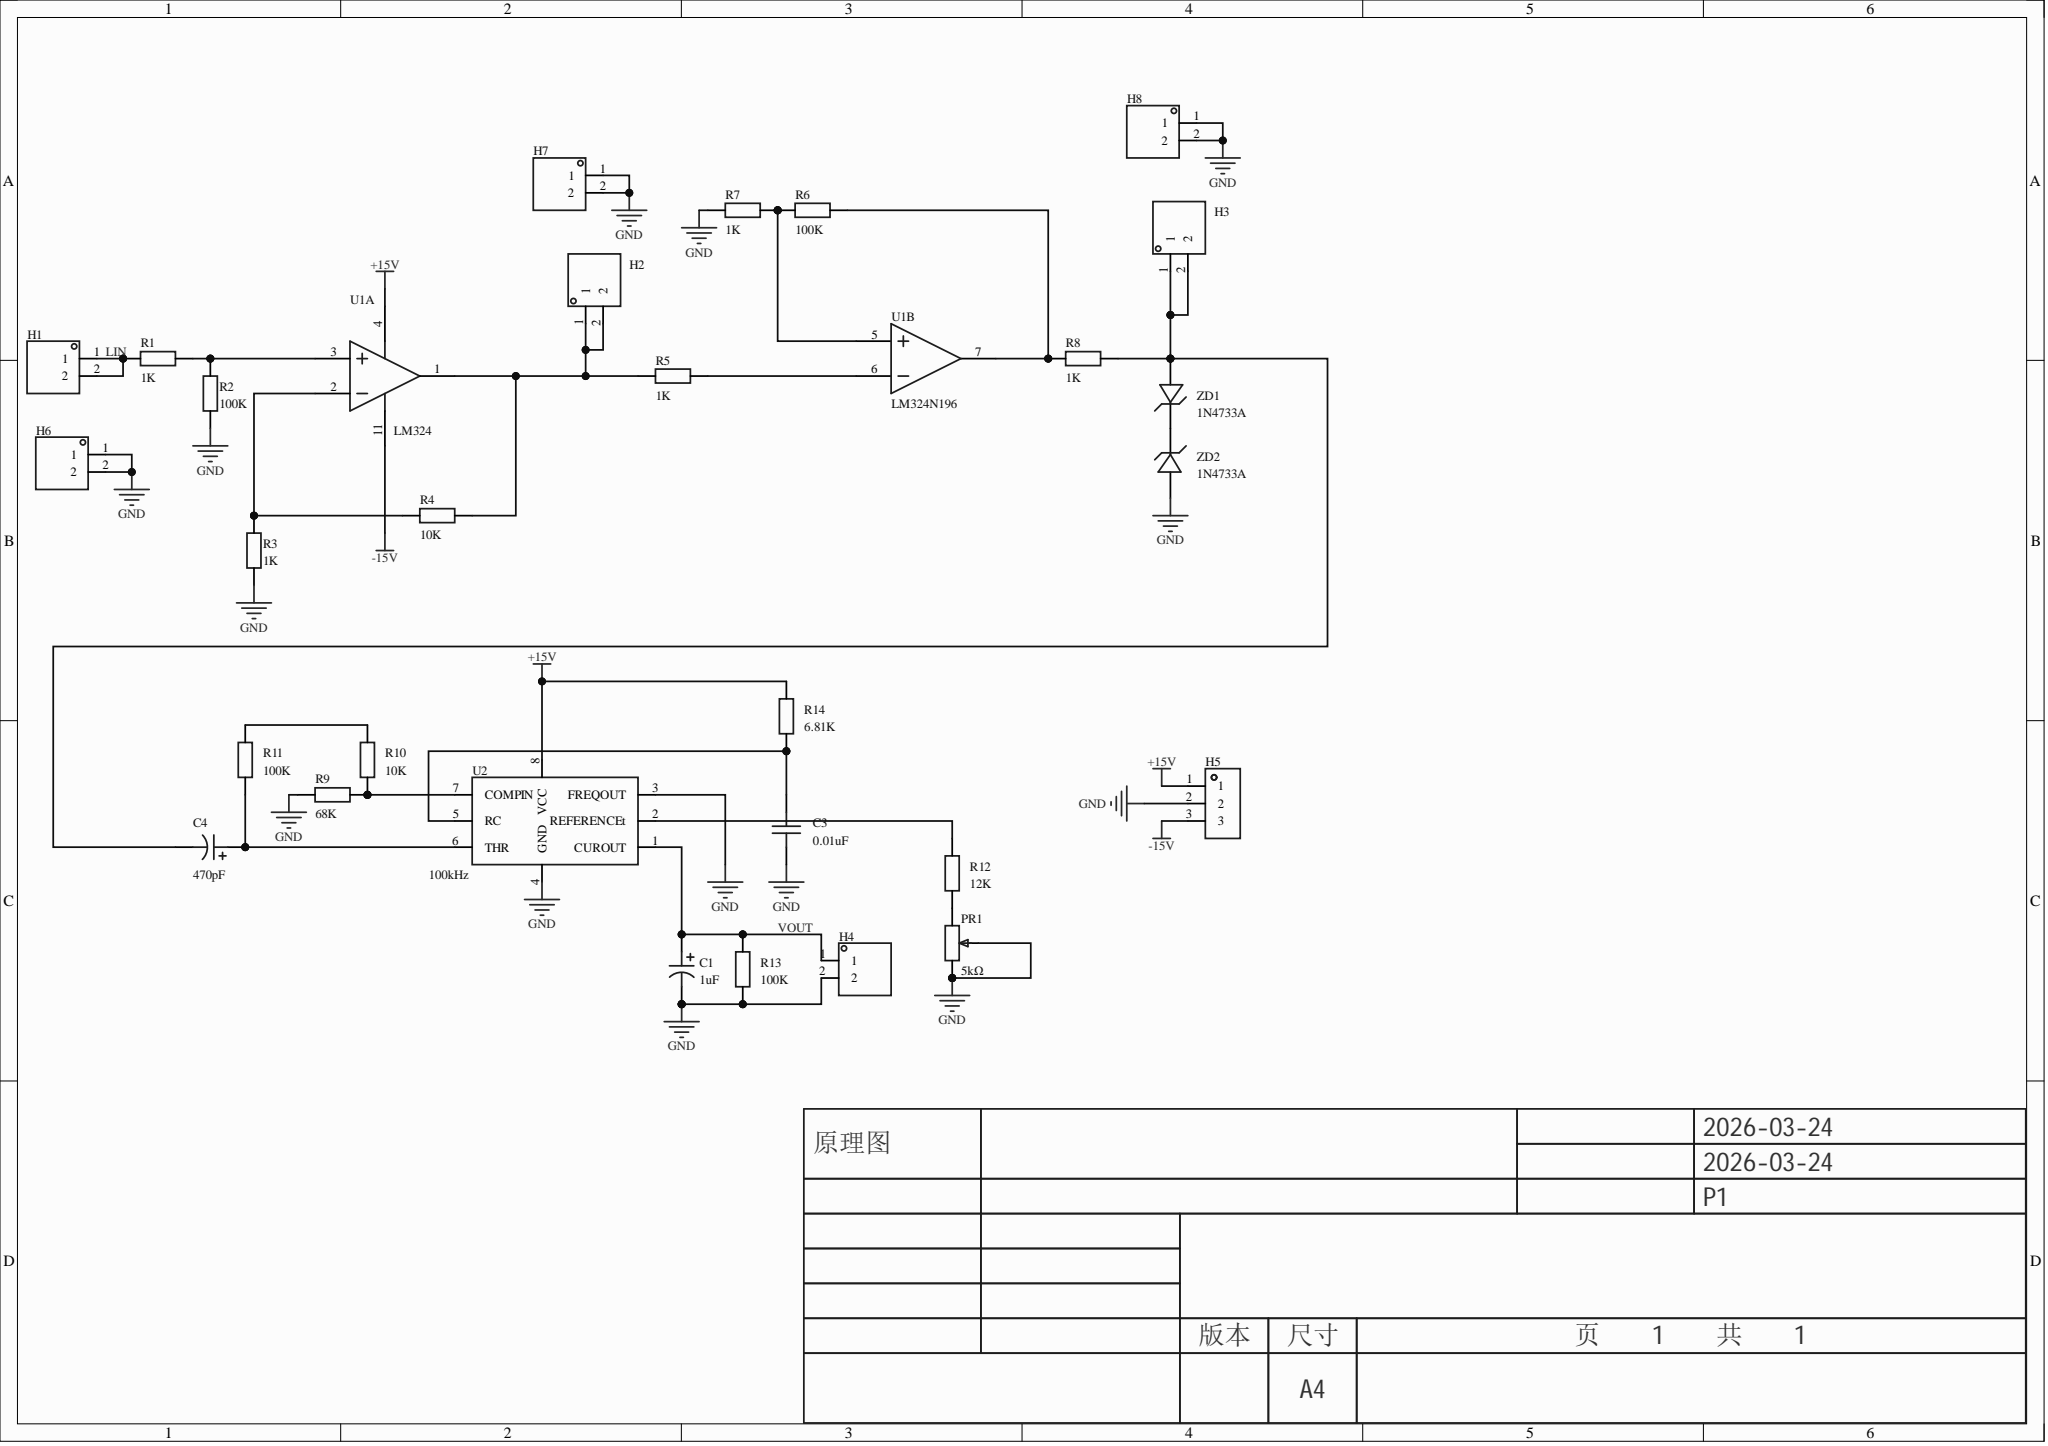Circuit board | Altium Designer | 30 parts | 19 nets
Bill of materials:
Comment,Description,Designator,Footprint,LibRef,Quantity
"1uF","","C1","CAP-TH_BD5.0-P2.00-D0.8-FD-10UF50VC110GL","10UF50VC110GL","1"
"0.01uF","","C3","C0805","CAP_0805","1"
"470pF","","C4","CAP-TH_BD5.0-P2.00-D0.8-FD-10UF50VC110GL","10UF50VC110GL","1"
"","","H1, H2, H3, H4, H6, H7, H8","HDR-TH_2P-P2.54-V-M-1","HDR-M_2.54_1x2P","7"
"","","H5","HDR-TH_3P-P2.54-V-M","HDR-M_2.54_1x3P","1"
"5kΩ","","PR1","R_3296","R_3296","1"
"1K","","R1, R3, R5, R7, R8","R0805","Res_0805","5"
"100K","","R2, R6, R11, R13","R0805","Res_0805","4"
"10K","","R4, R10","R0805","Res_0805","2"
"68K","","R9","R0805","Res_0805","1"
"12K","","R12","R0805","Res_0805","1"
"6.81K","","R14","R0805","Res_0805","1"
"LM324","","U1","PDIP-14_L19.3-W6.5-P2.54-LS7.6-BL","LM324N196","1"
"100kHz","","U2","DIP-8_L9.2-W6.4-P2.54-LS7.6-BL","LM331","1"
"1N4733A","","ZD1, ZD2","DO-41_BD2.8-L4.2-P8.00-D0.7-FD","1N4733A","2"
Netlist (Protel format):
[
C1
CAP-TH_BD5.0-P2.00-D0.8-FD-10UF50VC110GL
1uF



]
[
C3
C0805
0.01uF



]
[
C4
CAP-TH_BD5.0-P2.00-D0.8-FD-10UF50VC110GL
470pF



]
[
H1
HDR-TH_2P-P2.54-V-M-1




]
[
H2
HDR-TH_2P-P2.54-V-M-1




]
[
H3
HDR-TH_2P-P2.54-V-M-1




]
[
H4
HDR-TH_2P-P2.54-V-M-1




]
[
H5
HDR-TH_3P-P2.54-V-M




]
[
H6
HDR-TH_2P-P2.54-V-M-1




]
[
H7
HDR-TH_2P-P2.54-V-M-1




]
[
H8
HDR-TH_2P-P2.54-V-M-1




]
[
PR1
R_3296
5kΩ



]
[
R1
R0805
1K



]
[
R2
R0805
100K



]
[
R3
R0805
1K



]
[
R4
R0805
10K



]
[
R5
R0805
1K



]
[
R6
R0805
100K



]
[
R7
R0805
1K



]
[
R8
R0805
1K



]
[
R9
R0805
68K



]
[
R10
R0805
10K



]
[
R11
R0805
100K



]
[
R12
R0805
12K



]
[
R13
R0805
100K



]
[
R14
R0805
6.81K



]
[
U1
PDIP-14_L19.3-W6.5-P2.54-LS7.6-BL
LM324



]
[
U2
DIP-8_L9.2-W6.4-P2.54-LS7.6-BL
100kHz



]
[
ZD1
DO-41_BD2.8-L4.2-P8.00-D0.7-FD
1N4733A



]
[
ZD2
DO-41_BD2.8-L4.2-P8.00-D0.7-FD
1N4733A



]
(
VOUT
C1-1
H4-1
R13-2
U2-1
)
(
NetZD1_2
ZD1-2
ZD2-2
)
(
NetR12_2
R12-2
U2-2
)
(
NetR10_2
R10-2
R11-2
)
(
NetR9_2
R9-2
R10-1
U2-7
)
(
NetR6_2
R6-2
R7-1
U1-5
)
(
NetR6_1
R6-1
R8-2
U1-7
)
(
NetR5_1
R5-1
U1-6
)
(
NetR3_2
R3-2
R4-1
U1-2
)
(
NetR1_2
R1-2
R2-2
U1-3
)
(
NetPR1_3
PR1-3
R12-1
)
(
NetH2_1
H2-1
H2-2
R4-2
R5-2
U1-1
)
(
NetC4_2
C4-2
H3-1
H3-2
R8-1
ZD1-1
)
(
NetC4_1
C4-1
R11-1
U2-6
)
(
NetC3_2
C3-2
R14-1
U2-5
)
(
LIN
H1-1
H1-2
R1-1
)
(
GND
C1-2
C3-1
H4-2
H5-2
H6-1
H6-2
H7-1
H7-2
H8-1
H8-2
PR1-1
PR1-2
R2-1
R3-1
R7-2
R9-1
R13-1
U2-3
U2-4
ZD2-1
)
(
-15V
H5-3
U1-11
)
(
+15V
H5-1
R14-2
U1-4
U2-8
)